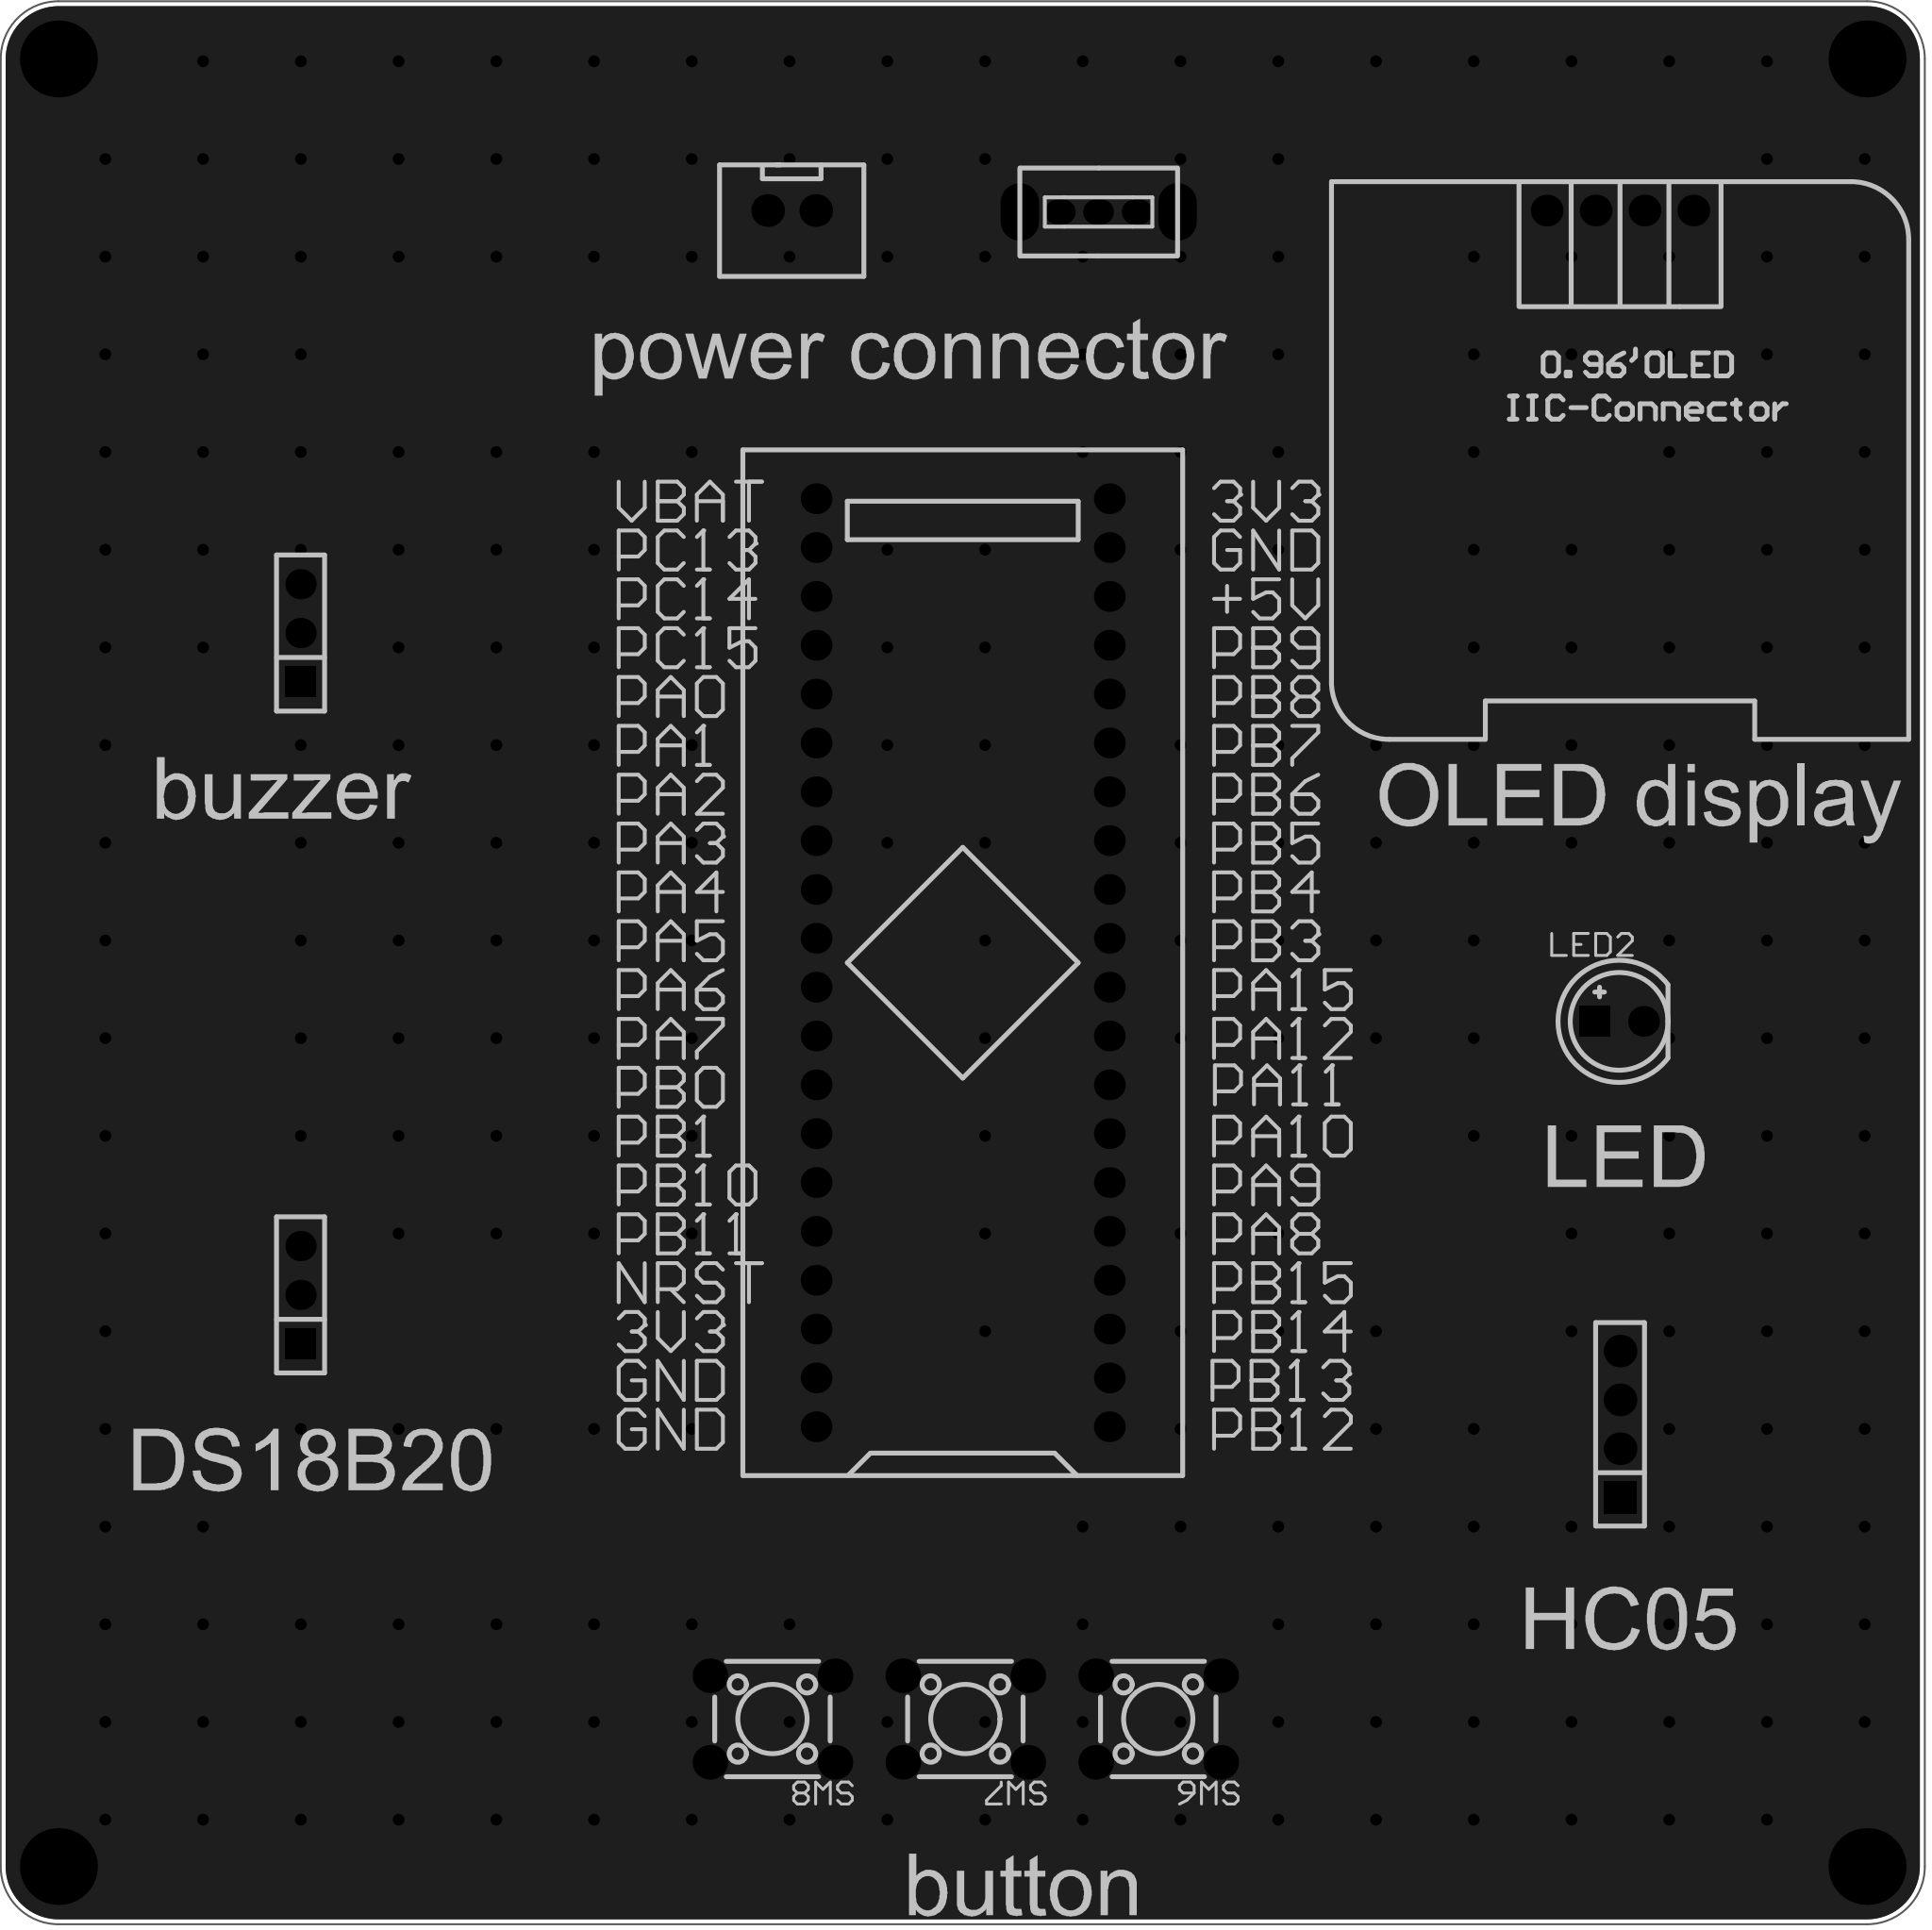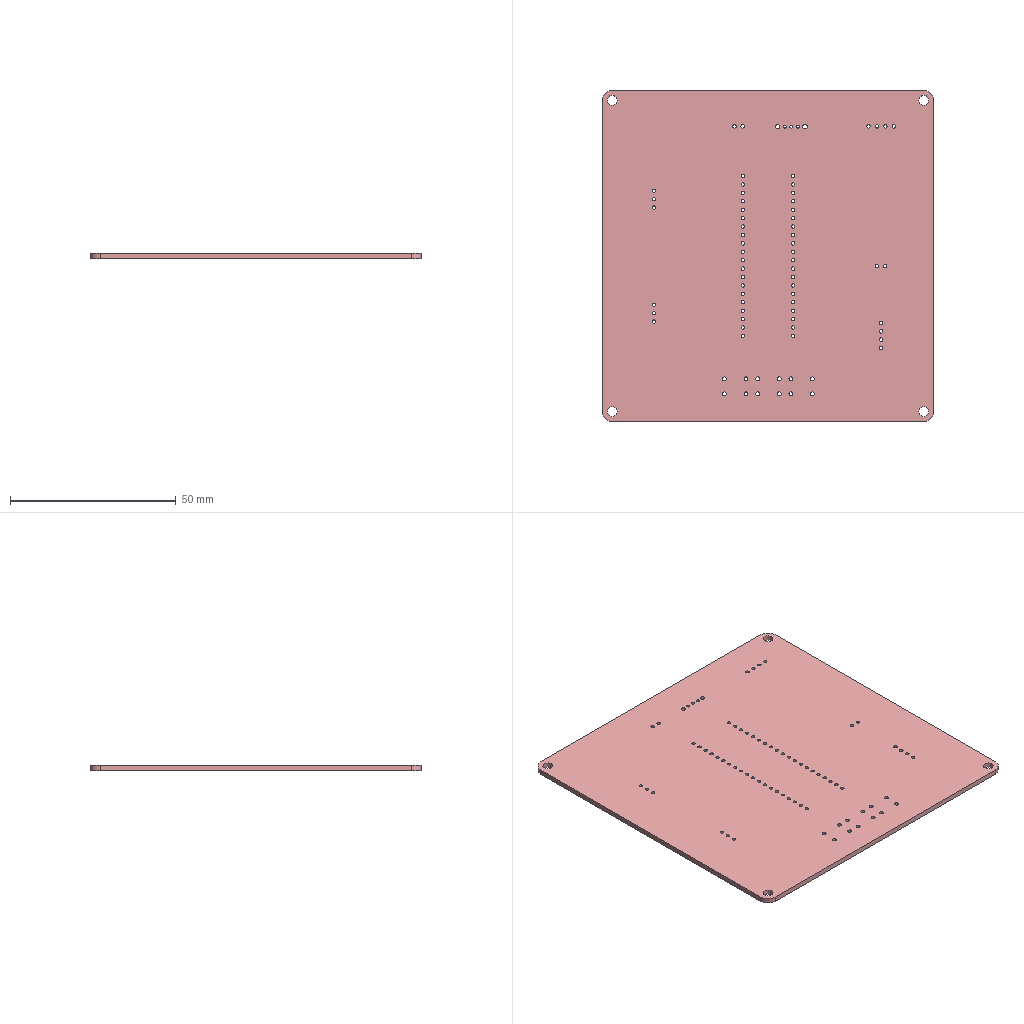Circuit board layout | Altium Designer | box 100 x 100 x 1.6 mm
Layer stack:
# Altium Designer layer stack of  (unit mm; dielectric type: 0 none, 1 core, 2 prepreg, 3 surface material)
index,name,kind,layer,copper_thickness_mm,dielectric_type,dielectric_thickness_mm,dielectric_material,dielectric_constant
0,Top Paste Mask Layer,other,,,,,,
1,Top Silkscreen Layer,other,,,,,,
2,Top Solder Mask Layer,dielectric,,,3,0.01,,3.3
3,Top Layer,copper,Top Layer,0.035,,,,
4,Dielectric1,dielectric,,,3,1.51,FR4,4.5
5,Bottom Layer,copper,Bottom Layer,0.035,,,,
6,Bottom Solder Mask Layer,dielectric,,,3,0.01,,3.3
7,Bottom Silkscreen Layer,other,,,,,,
8,Bottom Paste Mask Layer,other,,,,,,
# drill layer pairs: low layer,high layer
drill_pair,Top Layer,Bottom Layer
Part placement:
Designator,Comment,Layer,Footprint,Center-X(mm),Center-Y(mm),Rotation
U1,STM32F103C8T6-Card,TopLayer,CONN-TH_L53.3-W22.9_STM32F103C8T6-CARD,141.351,130.937,90
OLED1,,TopLayer,0.96OLED_4P,175.514,170.053,0
CN4,XH2.54*2P_THT,TopLayer,CONN-TH_2P-P2.50-XH2.54-2P,132.461,170.053,0
SW5,,TopLayer,拨动开关,148.417,169.978,0
H1,,TopLayer,HDR-TH_3P-P2.54-V-F,106.934,148.082,90
H2,,TopLayer,HDR-TH_4P-P2.54-V-F,175.514,106.934,90
H3,,TopLayer,HDR-TH_3P-P2.54-V-F,106.934,113.665,90
LED2,,TopLayer,LED-TH_5mm,175.464,127.889,0
SW6,,TopLayer,SW-TH_4P-L6.0-W6.0-P4.50-LS6.5,151.511,91.609,180
SW7,,TopLayer,SW-TH_4P-L6.0-W6.0-P4.50-LS6.5,141.485,91.609,180
SW8,,TopLayer,SW-TH_4P-L6.0-W6.0-P4.50-LS6.5,131.459,91.609,180
Pad and via stacks:
# Altium Designer via and pad stacks of  (unit mm). Each distinct definition once, with the count of objects using it.
# via: kind,start_layer,end_layer,hole_mm,diameter_mm,mode(0 simple;1 top-mid-bottom;2 full stack),diameter_per_layer,count,example_net
# pad: kind,layer,hole_mm,hole_type(0 round;1 square;2 slot),plating,top_size,top_shape(1 round;2 rect;3 octagon;9 rounded rect),mid_size,bottom_size,mode,footprint,size_per_layer,count,example
pad,Multi-Layer,3,0,plated,4x4,1,4x4,4x4,0,,,4,1
pad,Multi-Layer,1,0,plated,1.6x1.6,1,1.6x1.6,1.6x1.6,0,CONN-TH_L53.3-W22.9_STM32F103C8T6-CARD,,40,U1.1
pad,Multi-Layer,1,0,plated,1.65x1.65,1,1.65x1.65,1.65x1.65,0,0.96OLED_4P,,4,OLED1.4
pad,Multi-Layer,1.05,0,plated,1.7x1.7,1,1.7x1.7,1.7x1.7,0,CONN-TH_2P-P2.50-XH2.54-2P,,2,CN4.2
pad,Multi-Layer,0.8992,0,plated,1.6x1.3,1,1.6x1.3,1.6x1.3,0,\u00B2\u00A6\u00B6\u00AF\u00BF\u00AA\u00B9\u00D8,,3,SW5.1
pad,Multi-Layer,1.3,0,plated,3x1.999,1,3x1.999,3x1.999,0,\u00B2\u00A6\u00B6\u00AF\u00BF\u00AA\u00B9\u00D8,,2,SW5.4
pad,Multi-Layer,1.02,0,plated,1.575x1.575,1,1.575x1.575,1.575x1.575,0,HDR-TH_3P-P2.54-V-F,,4,H1.3
pad,Multi-Layer,1.02,0,plated,1.575x1.575,2,1.575x1.575,1.575x1.575,0,HDR-TH_3P-P2.54-V-F,,2,H1.1
pad,Multi-Layer,1.1,0,plated,1.7x1.7,2,1.7x1.7,1.7x1.7,0,HDR-TH_4P-P2.54-V-F,,1,H2.1
pad,Multi-Layer,1.1,0,plated,1.7x1.7,1,1.7x1.7,1.7x1.7,0,HDR-TH_4P-P2.54-V-F,,3,H2.2
pad,Multi-Layer,1,0,plated,1.6x1.6,2,1.6x1.6,1.6x1.6,0,LED-TH_5mm,,1,LED2.1
pad,Multi-Layer,1,0,plated,1.6x1.6,1,1.6x1.6,1.6x1.6,0,LED-TH_5mm,,1,LED2.2
pad,Multi-Layer,1.2,0,plated,1.8x1.8,1,1.8x1.8,1.8x1.8,0,SW-TH_4P-L6.0-W6.0-P4.50-LS6.5,,12,SW6.1
via,Top Layer,Bottom Layer,0.3048,0.61,0,,271,GND
Copper pours:
name,layer,net,type(0 solid;1 hatched;2 none)
Bottom Layer-GND,Bottom Layer,GND,0
Top Layer-GND,Top Layer,GND,0
Design rules, without the lines most boards share:
# Altium Designer design rules of  (exported by Altium Designer, unit mm)
# columns: name | kind | enabled | priority | scope1 | scope2 | descriptor | typed fields (field=value)
Copper_copperRegion_copperThickness1oz | 0 | disabled | 4 | All | All | Clearance Constraint (Gap=5.984mil) (Disabled)(All),(All) | gap=0.152
Copper_copperRegion_copperThickness1oz_1 | 63 | disabled | 4 | All | All | Board Clearance Constraint (Gap=0mil) (Disabled)(All) |
Copper_copperRegion_Copper_copperRegion | 0 | disabled | 5 | All | All | Clearance Constraint (Gap=5.984mil) (Disabled)(All),(All) | gap=0.152
Copper_copperRegion_Copper_copperRegion_1 | 63 | disabled | 5 | All | All | Board Clearance Constraint (Gap=0mil) (Disabled)(All) |
copperThickness1oz | 0 | enabled | 6 | All | All | Clearance Constraint (Gap=5.984mil) (All),(All) | gap=0.152
copperThickness1oz_1 | 63 | enabled | 6 | All | All | Board Clearance Constraint (Gap=0mil) (All) |
copperRegion_copperThickness1oz | 20 | disabled | 1 | All | All | Polygon Connect Rule(Relief Connect )(Conductor Width=10mil) (Relief Angle=90 Angle) (Entries=4) (Air Gap Width=10mil) (Disabled)(All),(All) | connect_style(0=relief,1=direct,2=none)=0 relief_conductor_width=0.254 relief_entries=4
copperRegion_Copper_copperRegion | 20 | disabled | 2 | All | All | Polygon Connect Rule(Relief Connect )(Conductor Width=10mil) (Relief Angle=90 Angle) (Entries=4) (Air Gap Width=10mil) (Disabled)(All),(All) | connect_style(0=relief,1=direct,2=none)=0 relief_conductor_width=0.254 relief_entries=4
copperRegion | 20 | enabled | 3 | All | All | Polygon Connect Rule(Relief Connect )(Conductor Width=10mil) (Relief Angle=90 Angle) (Entries=4) (Air Gap Width=10mil) (All),(All) | connect_style(0=relief,1=direct,2=none)=0 relief_conductor_width=0.254 relief_entries=4